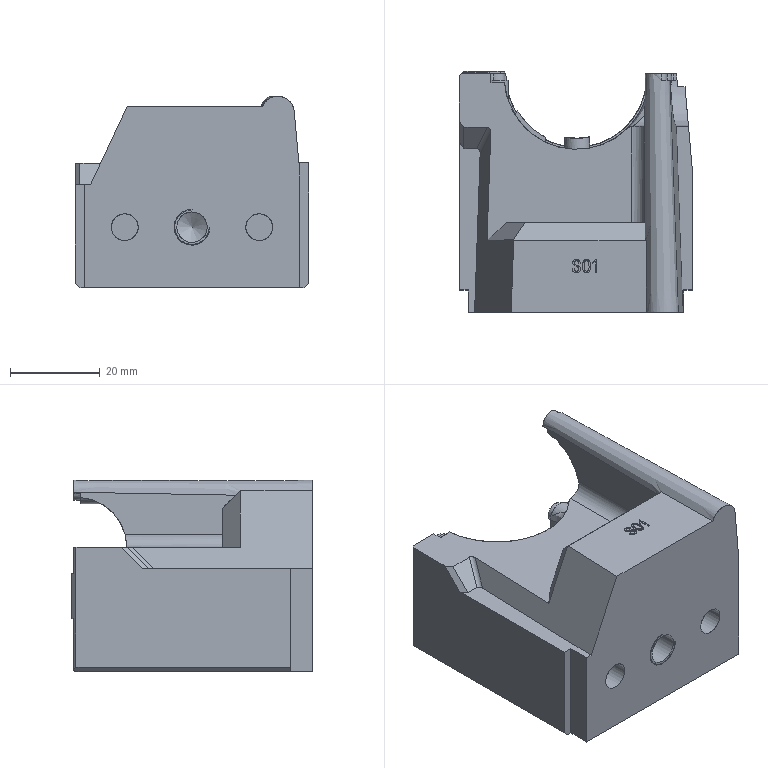NC program | PowerMill | posted with a generic post | part box 52 x 53.756 x 42.711 mm
Lines 1 to 924 of 9749:
%
O0001
N104 ( POWERMILL CB  : 2026004.0)
N105 ( POST VER      : 2026.0.0.5161)
N106 ( OPTION FILE   : FANUC)
N107 ( OUTPUT WORKPLANE : 2)
N108 (  )
N109 ( TOOL LIST )
N110 (----------------------------------)
N111 ( NO. | ID   | DIA.| TIP RAD|LENGTH)
N112 (----------------------------------)
N113 (    1|D6_1_1| 6.0 |  0.0   |114.16)
N114 (----------------------------------)
N115 (  )
N116 ( NUMBER OF TOOLPATHS: 1.0 )
N117 ( ESTIMATED PROGRAM DURATION: 0 HOURS 2 MIN 53 SEC)
N118 (  )
N119 G00 G21 G80 G40 G17
N120 G90
N121 G54
N122 G53 Z0.0
N123 (---------------)
N124 ( START TOOLPATH : 06开粗-D6-偏置区域二粗 )
N125 (---------------)
N126 ( TOOL NO.    :1 )
N127 ( TOOL TYPE   : ENDMILL)
N128 ( TOOL ID     : D6_1_1)
N129 ( TOOL DIA    : 6.0 LENGTH 114.16)
N130 T1
N131 M6
N132 S3800 M03
N133 G00 G90 X3.5472 Y27.6259
N134 G43 Z74.256 H1
N135
N136 G05 P10000 R8
N137 Z42.1845
N138 G01 Z39.1845 F2400.0
N139 X3.5456 Y27.616 F4000.0
N140 G03 X4.1895 Y25.9352 I1.7776 J-0.2827
N141 G01 X4.3126 Y25.8354
N142 X4.6394 Y25.4892
N143 X4.8959 Y25.1431
N144 X4.9344 Y25.0839
N145 X4.9815 Y25.0313
N146 G03 X5.5841 Y25.2972 I0.2426 J0.2659
N147 G01 X5.5845 Y27.9121
N148 X5.6031 Y28.086
N149 G03 X4.8735 Y29.7315 I-1.7899 J0.1909
N150 G01 X2.0879 Y28.641 Z39.0847
N151 X2.0881 Y28.631
N152 G03 X3.0207 Y27.0914 I1.7996 J0.0379
N153 G01 X3.2881 Y26.9445
N154 X3.6342 Y26.7087
N155 X3.8558 Y26.5276
N156 X4.2216 Y26.1815
N157 X4.5229 Y25.8354
N158 X4.6726 Y25.6414
N159 X4.7785 Y25.4892
N160 G03 X5.4346 Y25.6942 I0.2961 J0.2048
N161 G01 X5.4335 Y27.9121
N162 X5.4706 Y28.2582
N163 X5.547 Y28.6043
N164 X5.6664 Y28.9504
N165 X5.7103 Y29.0418
N166 G03 X5.5734 Y30.8366 I-1.6228 J0.7789
N167 G01 X1.2856 Y29.0778 Z38.9849
N168 X1.2865 Y29.0678
N169 G03 X2.3306 Y27.6016 I1.7919 J0.1711
N170 G01 X2.5959 Y27.4804
N171 X2.942 Y27.2896
N172 X3.2881 Y27.0657
N173 X3.5463 Y26.8737
N174 X3.9434 Y26.5276
N175 X4.2745 Y26.1815
N176 X4.5555 Y25.8354
N177 X4.6181 Y25.7458
N178 G03 X5.2732 Y25.952 I0.2951 J0.2061
N179 G01 X5.2731 Y26.1815
N180 X5.2823 Y27.9121
N181 X5.3198 Y28.2582
N182 X5.3959 Y28.6043
N183 X5.5154 Y28.9504
N184 X5.6679 Y29.2682
N185 G03 X5.5309 Y31.063 I-1.6228 J0.7787
N186 G01 X0.4554 Y29.2982 Z38.8851
N187 X0.4573 Y29.2884
N188 G03 X1.6352 Y27.9273 I1.7676 J0.3396
N189 G01 X1.9036 Y27.8342
N190 X2.2498 Y27.6912
N191 X2.505 Y27.5659
N192 X2.942 Y27.3177
N193 X3.2881 Y27.0833
N194 X3.5579 Y26.8737
N195 X3.9468 Y26.5276
N196 X4.2746 Y26.1815
N197 X4.4706 Y25.9399
N198 G03 X5.1101 Y26.1668 I0.2795 J0.2269
N199 G01 Y26.1815
N200 X5.1179 Y27.9121
N201 X5.1554 Y28.2582
N202 X5.2323 Y28.6043
N203 X5.3514 Y28.9504
N204 X5.518 Y29.2965
N205 X5.5634 Y29.3683
N206 G03 X5.6374 Y31.1668 I-1.5205 J0.9633
N207 G00 Z47.1845
N208 G01 X-5.6885 Y30.654 F10000.0
N209 G00 Z42.1845
N210 G01 Z39.1845 F2400.0
N211 X-5.6951 Y30.6464 F4000.0
N212 G03 X-6.0389 Y28.8796 I1.3583 J-1.1812
N213 G01 X-5.9442 Y28.6043
N214 X-5.8678 Y28.2582
N215 X-5.8304 Y27.9121
N216 X-5.8274 Y25.7959
N217 G03 X-5.1823 Y25.5765 I0.36 J0.0005
N218 G01 X-5.0187 Y25.7886
N219 X-4.6726 Y26.1496
N220 X-4.3265 Y26.4352
N221 X-4.1918 Y26.5276
N222 X-3.9804 Y26.656
N223 X-3.7608 Y26.7621
N224 G03 X-2.7487 Y28.2505 I-0.783 J1.6208
N225 G00 Z51.2768
N226 G01 X-25.8641 Y25.301 F10000.0
N227 G00 Z46.2768
N228 G01 Z43.2768 F2400.0
N229 X-25.8451 Y25.2136 F4000.0
N230 G03 X-25.6244 Y25.0715 I0.1814 J0.0393
N231 G01 X-25.4397 Y25.1115
N232 X-25.1489 Y25.1431
N233 X-23.363 Y25.1522
N234 X-19.2096 Y25.1525
N235 X-18.8634 Y25.1447
N236 X-14.71 Y25.1531
N237 X-14.246 Y25.1431
N238 X-13.6717 Y25.0692
N239 X-13.3255 Y24.9879
N240 X-12.9794 Y24.8719
N241 X-12.9145 Y24.8444
N242 G03 X-11.1283 Y25.0663 I0.7009 J1.6579
N243 G00 Z51.2768
N244 G01 X-11.6276 Y31.3456 F10000.0
N245 G00 Z46.2768
N246 G01 Z43.2768 F2400.0
N247 X-11.6367 Y31.3498 F4000.0
N248 G03 X-13.4283 Y31.1759 I-0.7452 J-1.6385
N249 G01 X-13.6365 Y31.0271
N250 X-14.0178 Y30.8213
N251 X-14.3845 Y30.681
N252 X-14.71 Y30.5967
N253 X-15.0561 Y30.5463
N254 X-15.4023 Y30.5343
N255 X-18.1712 Y30.531
N256 X-18.5173 Y30.5387
N257 X-19.2096 Y30.5312
N258 X-21.9785 Y30.5411
N259 X-22.3246 Y30.5793
N260 X-22.6707 Y30.6553
N261 X-23.0168 Y30.7754
N262 X-23.363 Y30.9421
N263 X-23.5053 Y31.0271
N264 X-23.7091 Y31.1645
N265 X-23.9619 Y31.3732
N266 X-24.0283 Y31.4361
N267 G03 X-25.7792 Y31.8539 I-1.2373 J-1.3073
N268 G00 Z51.177
N269 G01 X-25.64 Y25.9528 F10000.0
N270 G00 Z46.177
N271 G01 Z43.177 F2400.0
N272 X-25.4926 Y25.7206 F4000.0
N273 G03 X-25.718 Y25.218 I0.2681 J-0.4221
N274 G01 X-25.4397 Y25.2775
N275 X-25.0936 Y25.3113
N276 X-22.3246 Y25.3077
N277 X-19.5557
N278 X-19.2096 Y25.3152
N279 X-17.1328 Y25.3064
N280 X-14.3639 Y25.3108
N281 X-14.0178 Y25.288
N282 X-13.6717 Y25.2449
N283 X-13.3255 Y25.1735
N284 X-12.9794 Y25.0631
N285 X-12.7411 Y24.9668
N286 G03 X-10.9585 Y25.2167 I0.6748 J1.6687
N287 G00 Z51.177
N288 G01 X-11.5417 Y31.516 F10000.0
N289 G00 Z46.177
N290 G01 Z43.177 F2400.0
N291 X-11.5513 Y31.5189 F4000.0
N292 G03 X-13.3035 Y31.1067 I-0.5192 J-1.7235
N293 G01 X-13.3255 Y31.086
N294 X-13.6717 Y30.8422
N295 X-13.9706 Y30.681
N296 X-14.3639 Y30.5247
N297 X-14.71 Y30.4346
N298 X-15.0561 Y30.3835
N299 X-15.4023 Y30.3723
N300 X-17.8251 Y30.3775
N301 X-18.1712 Y30.3698
N302 X-19.5557 Y30.3761
N303 X-21.9785 Y30.3753
N304 X-22.3246 Y30.4119
N305 X-22.6707 Y30.4868
N306 X-23.0168 Y30.6039
N307 X-23.1911 Y30.681
N308 X-23.363 Y30.7683
N309 X-23.7091 Y30.989
N310 X-24.0552 Y31.2817
N311 X-24.1454 Y31.3732
N312 X-24.1604 Y31.3912
N313 G03 X-25.8515 Y32.0077 I-1.3795 J-1.1563
N314 G00 Z51.0772
N315 G01 X-25.7718 Y26.0953 F10000.0
N316 G00 Z46.0772
N317 G01 Z43.0772 F2400.0
N318 X-25.6178 Y25.8674 F4000.0
N319 G03 X-25.8286 Y25.3574 I0.2799 J-0.4142
N320 G01 X-25.7858 Y25.3714
N321 X-25.4397 Y25.4435
N322 X-25.0936 Y25.4763
N323 X-14.3639 Y25.4796
N324 X-14.0178 Y25.4661
N325 X-13.6717 Y25.4234
N326 X-13.3255 Y25.3617
N327 X-12.9794 Y25.2597
N328 X-12.6333 Y25.1259
N329 X-12.5882 Y25.1045
N330 G03 X-10.794 Y25.2489 I0.772 J1.626
N331 G00 Z51.0772
N332 G01 X-11.4271 Y31.3445 F10000.0
N333 G00 Z46.0772
N334 G01 Z43.0772 F2400.0
N335 X-11.4366 Y31.3478 F4000.0
N336 G03 X-13.2056 Y31.0153 I-0.5965 J-1.6983
N337 G01 X-13.3255 Y30.9124
N338 X-13.6522 Y30.681
N339 X-14.0178 Y30.4855
N340 X-14.4216 Y30.3349
N341 X-14.71 Y30.2624
N342 X-15.0561 Y30.2121
N343 X-15.4023 Y30.2008
N344 X-17.8251 Y30.209
N345 X-18.1712 Y30.2012
N346 X-21.9785 Y30.2041
N347 X-22.3246 Y30.2382
N348 X-22.6707 Y30.311
N349 X-23.0168 Y30.4258
N350 X-23.363 Y30.5875
N351 X-23.5242 Y30.681
N352 X-23.7091 Y30.8049
N353 X-23.9843 Y31.0271
N354 X-24.0552 Y31.0933
N355 X-24.2555 Y31.3094
N356 G03 X-25.9752 Y31.841 I-1.3202 J-1.2235
N357 G00 Z50.9773
N358 G01 X-25.8665 Y26.2488 F10000.0
N359 G00 Z45.9773
N360 G01 Z42.9773 F2400.0
N361 X-25.7045 Y26.0266 F4000.0
N362 G03 X-25.8978 Y25.5124 I0.2944 J-0.4042
N363 G01 X-25.7858 Y25.5487
N364 X-25.4397 Y25.6197
N365 X-25.0936 Y25.6518
N366 X-23.7091 Y25.6594
N367 X-19.2096 Y25.6596
N368 X-18.8634 Y25.6516
N369 X-16.0945 Y25.6591
N370 X-14.0178 Y25.6534
N371 X-13.6717 Y25.6158
N372 X-13.3255 Y25.5602
N373 X-13.0417 Y25.4892
N374 X-12.6333 Y25.3409
N375 X-12.4338 Y25.2486
N376 G03 X-10.6412 Y25.4112 I0.7555 J1.6338
N377 G01 X-11.326 Y31.3633
N378 X-11.3356 Y31.3662
N379 G03 X-13.0891 Y30.9596 I-0.5246 J-1.7218
N380 G01 X-13.3255 Y30.7387
N381 X-13.6717 Y30.4954
N382 X-13.9701 Y30.3349
N383 X-14.3639 Y30.1795
N384 X-14.71 Y30.0896
N385 X-15.0561 Y30.0407
N386 X-15.4023 Y30.0292
N387 X-17.1328 Y30.0252
N388 X-18.5173 Y30.0328
N389 X-19.2096 Y30.0238
N390 X-21.9785 Y30.0327
N391 X-22.3246 Y30.0645
N392 X-22.6707 Y30.1352
N393 X-23.0168 Y30.2476
N394 X-23.2199 Y30.3349
N395 X-23.363 Y30.4067
N396 X-23.7091 Y30.6208
N397 X-23.7907 Y30.681
N398 X-24.0552 Y30.9049
N399 X-24.1777 Y31.0271
N400 X-24.3656 Y31.2465
N401 G03 X-26.0632 Y31.8448 I-1.367 J-1.1711
N402 G01 X-25.2099 Y27.2279 Z42.8775
N403 X-24.9811 Y27.0753
N404 G02 X-25.799 Y26.1922 I-3.1646 J2.1105
N405 G03 X-25.9757 Y25.6777 I0.3084 J-0.3935
N406 G01 X-25.7858 Y25.7392
N407 X-25.4397 Y25.8089
N408 X-25.1776 Y25.8354
N409 X-19.5557 Y25.8374
N410 X-19.2096 Y25.8424
N411 X-18.8634 Y25.8375
N412 X-14.0178 Y25.8368
N413 X-13.6717 Y25.8082
N414 X-13.3255 Y25.7575
N415 X-12.9794 Y25.6778
N416 X-12.6333 Y25.5558
N417 X-12.2872 Y25.4078
N418 X-12.2695 Y25.3981
N419 G03 X-10.4699 Y25.4349 I0.8678 J1.5769
N420 G00 Z50.8775
N421 G01 X-11.2548 Y31.4773 F10000.0
N422 G00 Z45.8775
N423 G01 Z42.8775 F2400.0
N424 X-11.2646 Y31.4792 F4000.0
N425 G03 X-12.9668 Y30.894 I-0.3443 J-1.7668
N426 G01 X-12.9794 Y30.8795
N427 X-13.1796 Y30.681
N428 X-13.3255 Y30.5555
N429 X-13.6356 Y30.3349
N430 X-14.0178 Y30.1291
N431 X-14.39 Y29.9888
N432 X-14.71 Y29.9069
N433 X-15.0561 Y29.857
N434 X-15.4023 Y29.8468
N435 X-18.6904 Y29.8432
N436 X-21.9785 Y29.8461
N437 X-22.3246 Y29.8753
N438 X-22.6707 Y29.9438
N439 X-23.0168 Y30.0535
N440 X-23.363 Y30.2107
N441 X-23.5766 Y30.3349
N442 X-23.7091 Y30.4223
N443 X-24.0317 Y30.681
N444 X-24.3584 Y31.0271
N445 X-24.4849 Y31.205
N446 G03 X-26.1219 Y31.9535 I-1.4668 J-1.0434
N447 G00 Z50.7777
N448 G01 X-29.275 Y26.2697 F10000.0
N449 G00 Z45.7777
N450 G01 Z42.7777 F2400.0
N451 X-26.0 F4000.0
N452 Y25.8604
N453 X-25.7858 Y25.9296
N454 X-25.4397 Y25.9982
N455 X-25.0936 Y26.0286
N456 X-24.4013 Y26.0311
N457 X-14.0178 Y26.03
N458 X-13.6717 Y26.0113
N459 X-13.3255 Y25.9635
N460 X-12.9794 Y25.8974
N461 X-12.7592 Y25.8354
N462 X-12.6333 Y25.7909
N463 X-12.2872 Y25.6451
N464 X-12.1446 Y25.5709
N465 G03 X-10.3463 Y25.649 I0.8315 J1.5964
N466 G01 X-11.1746 Y31.4704
N467 X-11.1845 Y31.472
N468 G03 X-12.8633 Y30.8225 I-0.2769 J-1.7786
N469 G01 X-12.9794 Y30.6783
N470 X-13.3255 Y30.3552
N471 X-13.6717 Y30.1123
N472 X-13.8946 Y29.9888
N473 X-14.0178 Y29.9299
N474 X-14.3639 Y29.7974
N475 X-14.71 Y29.7085
N476 X-15.0561 Y29.6591
N477 X-15.4023 Y29.6492
N478 X-17.8251 Y29.6576
N479 X-18.1712 Y29.6496
N480 X-21.9785 Y29.6507
N481 X-22.3246 Y29.6778
N482 X-22.6707 Y29.744
N483 X-23.0168 Y29.8514
N484 X-23.3291 Y29.9888
N485 X-23.7091 Y30.2132
N486 X-23.873 Y30.3349
N487 X-24.0552 Y30.4889
N488 X-24.2479 Y30.681
N489 X-24.4013 Y30.8601
N490 X-24.5258 Y31.0271
N491 X-24.5734 Y31.1052
N492 G03 X-26.1533 Y31.9678 I-1.537 J-0.9369
N493 G00 Z50.6779
N494 G01 X-29.275 Y26.5284 F10000.0
N495 G00 Z45.6779
N496 G01 Z42.6779 F2400.0
N497 X-26.0 F4000.0
N498 Y26.0688
N499 X-25.7858 Y26.1367
N500 X-25.4397 Y26.2043
N501 X-25.0936 Y26.233
N502 X-23.7091 Y26.238
N503 X-19.2096 Y26.2382
N504 X-18.8634 Y26.2295
N505 X-18.1712 Y26.2365
N506 X-14.0178 Y26.2383
N507 X-13.6717 Y26.2289
N508 X-13.3166 Y26.1815
N509 X-12.9794 Y26.1207
N510 X-12.6333 Y26.026
N511 X-12.2872 Y25.8877
N512 X-11.9916 Y25.7366
N513 G03 X-10.1939 Y25.8286 I0.8192 J1.6028
N514 G01 X-11.1131 Y31.4796
N515 X-11.1231 Y31.4806
N516 G03 X-12.7634 Y30.7394 I-0.1782 J-1.7911
N517 G01 X-12.8053 Y30.681
N518 X-12.9794 Y30.4769
N519 X-13.1199 Y30.3349
N520 X-13.3255 Y30.1548
N521 X-13.5523 Y29.9888
N522 X-13.6717 Y29.9125
N523 X-14.0178 Y29.7307
N524 X-14.2362 Y29.6427
N525 X-14.3639 Y29.5986
N526 X-14.71 Y29.5102
N527 X-15.0561 Y29.4612
N528 X-15.4023 Y29.4516
N529 X-16.7867 Y29.447
N530 X-18.8634 Y29.4556
N531 X-19.2096 Y29.4455
N532 X-21.9785 Y29.4522
N533 X-22.3246 Y29.4777
N534 X-22.6707 Y29.5417
N535 X-23.0168 Y29.6469
N536 X-23.363 Y29.7979
N537 X-23.7091 Y30.0023
N538 X-24.0552 Y30.2743
N539 X-24.1205 Y30.3349
N540 X-24.4013 Y30.6394
N541 X-24.6717 Y31.0271
N542 X-24.6883 Y31.0562
N543 G03 X-26.2416 Y31.9657 I-1.5643 J-0.8905
N544 G01 X-29.275 Y26.8171 Z42.5781
N545 X-26.0
N546 Y26.2863
N547 X-25.7858 Y26.3538
N548 X-25.4397 Y26.4212
N549 X-25.0936 Y26.4498
N550 X-24.7474 Y26.4434
N551 X-19.5557 Y26.4452
N552 X-19.2096 Y26.4516
N553 X-17.8251 Y26.4407
N554 X-13.6717 Y26.4444
N555 X-13.3255 Y26.4087
N556 X-12.9794 Y26.3531
N557 X-12.6333 Y26.2691
N558 X-12.2872 Y26.1428
N559 X-11.9411 Y25.9708
N560 X-11.8518 Y25.9196
N561 G03 X-10.0518 Y25.9243 I0.8959 J1.5612
N562 G01 X-10.971 Y31.398
N563 X-10.9809 Y31.3992
N564 G03 X-12.639 Y30.6985 I-0.2223 J-1.7862
N565 G01 X-12.9139 Y30.3349
N566 X-12.9794 Y30.262
N567 X-13.3255 Y29.9393
N568 X-13.6717 Y29.6969
N569 X-14.0178 Y29.5144
N570 X-14.3639 Y29.383
N571 X-14.7038 Y29.2965
N572 X-15.0561 Y29.2468
N573 X-15.4023 Y29.237
N574 X-15.7484 Y29.2429
N575 X-17.8251 Y29.2408
N576 X-18.1712 Y29.2322
N577 X-21.6324 Y29.242
N578 X-21.9785 Y29.2333
N579 X-22.3246 Y29.2568
N580 X-22.6707 Y29.3175
N581 X-23.0168 Y29.4203
N582 X-23.363 Y29.5685
N583 X-23.5025 Y29.6427
N584 X-23.7091 Y29.7684
N585 X-24.0552 Y30.0358
N586 X-24.3505 Y30.3349
N587 X-24.6127 Y30.681
N588 X-24.7474 Y30.9048
N589 X-24.7905 Y30.9876
N590 G03 X-26.3083 Y31.9553 I-1.597 J-0.8305
N591 G01 X-29.275 Y27.1187 Z42.4783
N592 X-26.0
N593 Y26.5132
N594 X-25.7858 Y26.5797
N595 X-25.4397 Y26.6465
N596 X-25.0936 Y26.6727
N597 X-24.4013 Y26.676
N598 X-19.5557 Y26.677
N599 X-13.6717 Y26.6752
N600 X-13.3255 Y26.6527
N601 X-12.9794 Y26.5984
N602 X-12.6463 Y26.5276
N603 X-12.2872 Y26.4108
N604 X-11.9411 Y26.2499
N605 X-11.6977 Y26.114
N606 G03 X-9.8979 Y26.1402 I0.8773 J1.5718
N607 G01 X-10.9531 Y31.5105
N608 X-10.9631 Y31.5106
N609 G03 X-12.5352 Y30.6341 I-0.027 J-1.7998
N610 G01 X-12.6333 Y30.47
N611 X-12.7269 Y30.3349
N612 X-12.9794 Y30.0269
N613 X-13.3255 Y29.7054
N614 X-13.6717 Y29.4639
N615 X-13.9875 Y29.2965
N616 X-14.3639 Y29.1509
N617 X-14.71 Y29.0632
N618 X-15.0561 Y29.0151
N619 X-15.4023 Y29.0065
N620 X-17.8251 Y29.0142
N621 X-18.1712 Y29.008
N622 X-21.9785 Y29.0084
N623 X-22.3246 Y29.0291
N624 X-22.6707 Y29.0877
N625 X-23.0168 Y29.1873
N626 X-23.363 Y29.332
N627 X-23.7091 Y29.5289
N628 X-23.8709 Y29.6427
N629 X-24.0552 Y29.791
N630 X-24.2625 Y29.9888
N631 X-24.4013 Y30.1423
N632 X-24.5519 Y30.3349
N633 X-24.7474 Y30.6378
N634 X-24.8807 Y30.9127
N635 G03 X-26.3705 Y31.9229 I-1.6198 J-0.7851
N636 G01 X-29.275 Y27.4435 Z42.3785
N637 X-26.0
N638 Y26.7613
N639 X-25.7858 Y26.8268
N640 X-25.4397 Y26.8923
N641 X-25.0936 Y26.9198
N642 X-24.7474 Y26.9148
N643 X-23.363 Y26.9197
N644 X-19.2096 Y26.9194
N645 X-18.8634 Y26.9089
N646 X-13.6717 Y26.9203
N647 X-13.3255 Y26.9073
N648 X-13.0616 Y26.8737
N649 X-12.6333 Y26.7866
N650 X-12.2872 Y26.6854
N651 X-11.9214 Y26.5276
N652 X-11.595 Y26.3462
N653 X-11.5724 Y26.3316
N654 G03 X-9.7748 Y26.2391 I0.979 J1.5105
N655 G01 X-10.9049 Y31.5502
N656 X-10.9149 Y31.5498
N657 G03 X-12.436 Y30.5874 I0.0729 J-1.7985
N658 G01 X-12.5685 Y30.3349
N659 X-12.6333 Y30.2315
N660 X-12.8075 Y29.9888
N661 X-12.9794 Y29.7879
N662 X-13.1239 Y29.6427
N663 X-13.3255 Y29.4664
N664 X-13.56 Y29.2965
N665 X-13.6717 Y29.2252
N666 X-14.0178 Y29.0434
N667 X-14.2523 Y28.9504
N668 X-14.3639 Y28.9128
N669 X-14.71 Y28.8247
N670 X-15.0561 Y28.778
N671 X-15.4023 Y28.7696
N672 X-18.1712 Y28.7628
N673 X-18.5173 Y28.7707
N674 X-19.2096 Y28.7641
N675 X-20.594 Y28.7682
N676 X-21.9785 Y28.768
N677 X-22.3246 Y28.7852
N678 X-22.6707 Y28.8406
N679 X-23.0168 Y28.9375
N680 X-23.363 Y29.0799
N681 X-23.7091 Y29.2736
N682 X-24.0552 Y29.5312
N683 X-24.1781 Y29.6427
N684 X-24.4013 Y29.8767
N685 X-24.4938 Y29.9888
N686 X-24.7311 Y30.3349
N687 X-24.9108 Y30.681
N688 X-24.981 Y30.8637
N689 G03 X-26.3803 Y31.996 I-1.6802 J-0.6457
N690 G01 X-29.275 Y27.8176 Z42.2787
N691 X-26.0
N692 Y27.0214
N693 X-25.7858 Y27.0859
N694 X-25.4397 Y27.1503
N695 X-25.0936 Y27.1749
N696 X-19.5557 Y27.1729
N697 X-19.2096 Y27.1804
N698 X-18.1712 Y27.1803
N699 X-17.8251 Y27.171
N700 X-13.3255 Y27.1654
N701 X-12.9794 Y27.1291
N702 X-12.6333 Y27.0644
N703 X-12.2872 Y26.9754
N704 X-11.9411 Y26.8417
N705 X-11.595 Y26.66
N706 X-11.4403 Y26.5631
N707 G03 X-9.6414 Y26.4978 I0.956 J1.5251
N708 G01 X-10.8796 Y31.6386
N709 X-10.8895 Y31.6374
N710 G03 X-12.3289 Y30.5566 I0.2163 J-1.7869
N711 G01 X-12.4235 Y30.3349
N712 X-12.6166 Y29.9888
N713 X-12.8708 Y29.6427
N714 X-12.9794 Y29.5195
N715 X-13.2088 Y29.2965
N716 X-13.3255 Y29.1985
N717 X-13.6852 Y28.9504
N718 X-14.0178 Y28.7768
N719 X-14.3639 Y28.6464
N720 X-14.5149 Y28.6043
N721 X-14.71 Y28.559
N722 X-15.0561 Y28.5126
N723 X-15.4023 Y28.5039
N724 X-17.8251 Y28.5153
N725 X-18.1712 Y28.5027
N726 X-19.2096 Y28.5018
N727 X-19.5557 Y28.5106
N728 X-21.9785 Y28.5053
N729 X-22.3246 Y28.5199
N730 X-22.6707 Y28.5725
N731 X-23.0168 Y28.666
N732 X-23.363 Y28.8042
N733 X-23.7091 Y28.9935
N734 X-24.0552 Y29.2446
N735 X-24.4013 Y29.5826
N736 X-24.706 Y29.9888
N737 X-24.8981 Y30.3349
N738 X-25.0413 Y30.681
N739 X-25.0754 Y30.7974
N740 G03 X-26.3775 Y32.0403 I-1.7274 J-0.5061
N741 G00 Z50.6332
N742 G01 X-10.8916 Y31.7644 F10000.0
N743 G00 Z45.1788
N744 G01 Z42.1788 F2400.0
N745 X-10.9014 Y31.7622 F4000.0
N746 G03 X-12.23 Y30.5478 I0.3875 J-1.7578
N747 G01 X-12.2872 Y30.3671
N748 X-12.4542 Y29.9888
N749 X-12.6333 Y29.6801
N750 X-12.9273 Y29.2965
N751 X-12.9794 Y29.239
N752 X-13.2871 Y28.9504
N753 X-13.6717 Y28.6785
N754 X-14.0178 Y28.4974
N755 X-14.3639 Y28.3677
N756 X-14.71 Y28.2807
N757 X-14.8595 Y28.2582
N758 X-15.0561 Y28.2357
N759 X-15.4023 Y28.2278
N760 X-18.1712 Y28.2219
N761 X-18.8634 Y28.2336
N762 X-19.2096 Y28.2198
N763 X-21.2863 Y28.2295
N764 X-21.9785 Y28.227
N765 X-22.3246 Y28.2389
N766 X-22.6707 Y28.29
N767 X-23.0168 Y28.3797
N768 X-23.363 Y28.5146
N769 X-23.7091 Y28.6992
N770 X-24.0591 Y28.9504
N771 X-24.4013 Y29.2771
N772 X-24.6857 Y29.6427
N773 X-24.7474 Y29.7371
N774 X-24.8883 Y29.9888
N775 X-25.04 Y30.3349
N776 X-25.0936 Y30.4884
N777 X-25.1488 Y30.681
N778 X-25.1723 Y30.7917
N779 G03 X-26.3761 Y32.1299 I-1.7609 J-0.3734
N780 G01 X-29.275 Y28.2286
N781 X-26.0
N782 Y27.3084
N783 X-25.7858 Y27.3738
N784 X-25.4397 Y27.4359
N785 X-25.0936 Y27.4612
N786 X-24.7474 Y27.4569
N787 X-23.363 Y27.4638
N788 X-19.2096 Y27.4641
N789 X-18.8634 Y27.4504
N790 X-18.1712 Y27.4603
N791 X-13.3255 Y27.462
N792 X-12.9794 Y27.4368
N793 X-12.6333 Y27.3734
N794 X-12.2872 Y27.2861
N795 X-11.9411 Y27.1683
N796 X-11.595 Y26.9998
N797 X-11.31 Y26.8221
N798 G03 X-9.511 Y26.7614 I0.9521 J1.5276
N799 G00 Z50.079
N800 G01 X-29.275 Y28.7185 F10000.0
N801 G00 Z45.079
N802 G01 Z42.079 F2400.0
N803 X-26.0 F4000.0
N804 Y27.6197
N805 X-25.7858 Y27.6828
N806 X-25.4397 Y27.7455
N807 X-25.0936 Y27.7683
N808 X-24.7474 Y27.7603
N809 X-19.5557 Y27.7615
N810 X-19.2096 Y27.774
N811 X-18.1712 Y27.773
N812 X-17.8251 Y27.7584
N813 X-13.3255 Y27.7613
N814 X-12.9794 Y27.748
N815 X-12.6333 Y27.6961
N816 X-12.2872 Y27.6224
N817 X-11.9411 Y27.5155
N818 X-11.595 Y27.3636
N819 X-11.3437 Y27.2198
N820 X-11.2085 Y27.1251
N821 G03 X-9.4154 Y26.9673 I1.0332 J1.4739
N822 G01 X-10.9028 Y31.8909
N823 X-10.9124 Y31.888
N824 G03 X-12.1422 Y30.5736 I0.5234 J-1.7223
N825 G01 X-12.1977 Y30.3349
N826 X-12.2872 Y30.0547
N827 X-12.4695 Y29.6427
N828 X-12.6333 Y29.3619
N829 X-12.9518 Y28.9504
N830 X-13.3255 Y28.6
N831 X-13.6717 Y28.36
N832 X-13.8554 Y28.2582
N833 X-14.0178 Y28.1802
N834 X-14.3639 Y28.0509
N835 X-14.71 Y27.9646
N836 X-15.0561 Y27.9192
N837 X-15.4023 Y27.9119
N838 X-15.7484 Y27.9217
N839 X-17.8251 Y27.9238
N840 X-18.1421 Y27.9121
N841 X-19.2096 Y27.9095
N842 X-19.5557 Y27.9222
N843 X-21.6324 Y27.9224
N844 X-21.9785 Y27.9141
N845 X-22.3246 Y27.922
N846 X-22.6707 Y27.9678
N847 X-23.0168 Y28.0555
N848 X-23.363 Y28.186
N849 X-23.7091 Y28.3664
N850 X-24.0504 Y28.6043
N851 X-24.4013 Y28.93
N852 X-24.6944 Y29.2965
N853 X-24.9015 Y29.6427
N854 X-25.0569 Y29.9888
N855 X-25.169 Y30.3349
N856 X-25.2445 Y30.681
N857 X-25.2576 Y30.7869
N858 G03 X-26.3426 Y32.2231 I-1.7863 J-0.2216
N859 G01 X-29.275 Y29.2648 Z41.9792
N860 X-26.0
N861 Y27.9734
N862 X-25.7858 Y28.0371
N863 X-25.4397 Y28.0982
N864 X-25.0936 Y28.121
N865 X-24.8123 Y28.1198
N866 G03 X-24.5281 Y28.7027 I0.0015 J0.36
N867 G01 X-24.7233 Y28.9504
N868 X-24.9301 Y29.2965
N869 X-25.0842 Y29.6427
N870 X-25.1959 Y29.9888
N871 X-25.2714 Y30.3349
N872 X-25.3159 Y30.681
N873 X-25.3262 Y30.9016
N874 G03 X-26.2985 Y32.4165 I-1.798 J-0.0846
N875 G01 X-29.275 Y29.9557 Z41.8794
N876 X-26.0
N877 Y28.3624
N878 X-25.7858 Y28.4251
N879 X-25.4397 Y28.4848
N880 X-25.3159 Y28.4929
N881 G03 X-25.0084 Y28.9937 I-0.0235 J0.3592
N882 G01 X-25.1379 Y29.2965
N883 X-25.2436 Y29.6427
N884 X-25.3143 Y29.9888
N885 X-25.3531 Y30.3349
N886 X-25.3665 Y30.681
N887 X-25.3554 Y31.0271
N888 X-25.1806 Y33.0233
N889 G03 X-25.9413 Y34.6547 I-1.7932 J0.157
N890 G01 X-29.275 Y30.9564 Z41.7796
N891 X-26.0
N892 Y28.8548
N893 X-25.7858 Y28.9165
N894 X-25.6197 Y28.9451
N895 G03 X-25.3253 Y29.3566 I-0.0611 J0.3548
N896 G01 X-25.3709 Y29.6427
N897 X-25.3982 Y29.9888
N898 X-25.4031 Y30.3349
N899 X-25.3895 Y30.681
N900 X-25.1741 Y33.1411
N901 G03 X-25.9346 Y34.7726 I-1.7931 J0.1571
N902 G01 X-29.275 Y32.1144 Z41.6798
N903 X-26.0
N904 Y29.5216
N905 X-25.7858 Y29.5842
N906 X-25.7165 Y29.5977
N907 X-25.6503 Y29.6218
N908 G03 X-25.4467 Y29.9402 I-0.1563 J0.3243
N909 G01 X-25.4459 Y29.9888
N910 X-25.423 Y30.3349
N911 X-25.1719 Y33.2027
N912 G03 X-25.9325 Y34.8341 I-1.7931 J0.157
N913 G01 X-29.275 Y32.1665 Z41.58
N914 X-26.0
N915 Y30.8876
N916 X-25.7858 Y30.9433
N917 X-25.6342 Y30.9721
N918 G03 X-25.3429 Y31.2943 I-0.0673 J0.3537
N919 G01 X-25.1724 Y33.2403
N920 G03 X-25.9329 Y34.8717 I-1.7931 J0.157
N921 G01 X-29.275 Y32.195 Z41.4802
N922 X-26.0
N923 Y30.9649
N924 X-25.7749 Y31.0271
N925 X-25.6455 Y31.0463
N926 G03 X-25.3397 Y31.371 I-0.0529 J0.3561
N927 G01 X-25.174 Y33.2621
N928 G03 X-25.9346 Y34.8935 I-1.7932 J0.1571
N929 G01 X-29.275 Y32.2077 Z41.3804
N930 X-26.0
N931 Y30.9719
N932 X-25.7987 Y31.0271
N933 X-25.6486 Y31.0495
N934 G03 X-25.3429 Y31.3741 I-0.053 J0.356
N935 G01 X-25.1768 Y33.2697
N936 G03 X-25.9373 Y34.9012 I-1.7932 J0.1571
N937 G01 X-29.275 Y32.2185 Z41.2805
N938 X-26.0
N939 Y30.9746
N940 X-25.8075 Y31.0271
N941 X-25.6524 Y31.0501
N942 G03 X-25.3464 Y31.3748 I-0.0526 J0.3561
N943 G01 X-25.1799 Y33.2747
N944 G03 X-25.9404 Y34.9062 I-1.7931 J0.1572
N945 G01 X-29.275 Y32.2281 Z41.1807
N946 X-26.0
N947 Y30.9772
N948 X-25.8162 Y31.0271
N949 X-25.656 Y31.0507
N950 G03 X-25.3498 Y31.3754 I-0.0524 J0.3562
N951 G01 X-25.183 Y33.2784
N952 G03 X-25.9435 Y34.9099 I-1.7931 J0.1571
N953 G01 X-29.275 Y32.241 Z41.0809
N954 X-26.0
N955 Y30.9798
N956 X-25.825 Y31.0271
N957 X-25.6598 Y31.0513
N958 G03 X-25.3533 Y31.3761 I-0.0521 J0.3562
N959 G01 X-25.1859 Y33.2858
N960 G03 X-25.9464 Y34.9173 I-1.7931 J0.1572
N961 G01 X-29.275 Y32.2511 Z40.9811
N962 X-26.0
N963 Y30.9824
N964 X-25.8337 Y31.0271
N965 X-25.6635 Y31.0519
N966 G03 X-25.3566 Y31.3767 I-0.0517 J0.3562
N967 G01 X-25.1889 Y33.2906
N968 G03 X-25.9494 Y34.922 I-1.7931 J0.1571
N969 G01 X-29.275 Y32.2611 Z40.8813
N970 X-26.0
N971 Y30.985
N972 X-25.8424 Y31.0271
N973 X-25.6672 Y31.0525
N974 G03 X-25.3601 Y31.3773 I-0.0515 J0.3562
N975 G01 X-25.1921 Y33.2945
N976 G03 X-25.9525 Y34.926 I-1.7931 J0.1572
N977 G01 X-29.275 Y32.2711 Z40.7815
N978 X-26.0
N979 Y30.9876
N980 X-25.8512 Y31.0271
N981 X-25.6709 Y31.053
N982 G03 X-25.3635 Y31.3779 I-0.0512 J0.3564
N983 G01 X-25.1951 Y33.2987
N984 G03 X-25.9556 Y34.9302 I-1.7931 J0.1572
N985 G01 X-29.275 Y32.2813 Z40.6817
N986 X-26.0
N987 Y30.9901
N988 X-25.8599 Y31.0271
N989 X-25.6747 Y31.0536
N990 G03 X-25.367 Y31.3785 I-0.0509 J0.3564
N991 G01 X-25.1983 Y33.3028
N992 G03 X-25.9587 Y34.9343 I-1.7931 J0.1572
N993 G01 X-29.275 Y32.2915 Z40.5819
N994 X-26.0
N995 Y30.9908
N996 X-25.9518 Y31.0028
N997 X-25.8599 Y31.0271
N998 X-25.8442 Y31.0299
N999 X-25.8287 Y31.0334
N1000 X-25.7858 Y31.044
N1001 X-25.6826 Y31.0573
N1002 G03 X-25.37 Y31.3829 I-0.0461 J0.3571
N1003 G01 X-25.2013 Y33.3072
N1004 G03 X-25.9618 Y34.9387 I-1.7932 J0.1572
N1005 G01 X-29.275 Y32.3017 Z40.4821
N1006 X-26.0
N1007 Y30.9931
N1008 X-25.7858 Y31.0457
N1009 X-25.6868 Y31.0582
N1010 G03 X-25.3734 Y31.3839 I-0.0452 J0.3572
N1011 G01 X-25.2044 Y33.3116
N1012 G03 X-25.9648 Y34.9431 I-1.7931 J0.1572
N1013 G01 X-29.275 Y32.3118 Z40.3823
N1014 X-26.0
N1015 Y30.9953
N1016 X-25.7858 Y31.0473
N1017 X-25.691 Y31.0591
N1018 G03 X-25.3768 Y31.385 I-0.0444 J0.3573
N1019 G01 X-25.2079 Y33.3145
N1020 G03 X-25.9685 Y34.9459 I-1.7931 J0.157
N1021 G01 X-29.275 Y32.322 Z40.2824